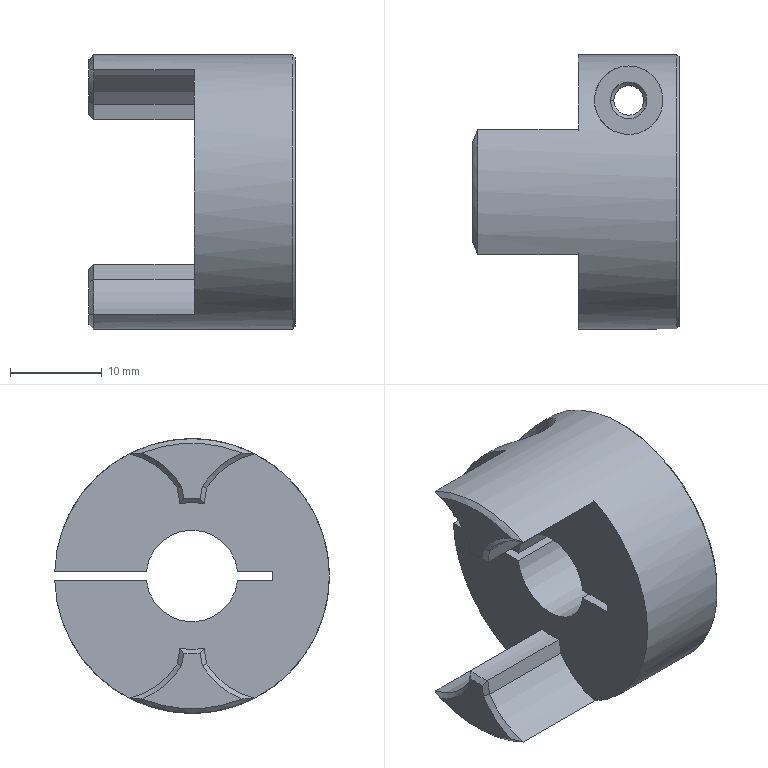Part | NX | 1 solid | 48 faces | box 22.5 x 29.992 x 30 mm | volume 7346 mm3 | plane 18 | cylinder 17 | cone 13 | commonest cylinder face diameters 4 x4 16.982 x4 3.242 x2 7.5 x2 10 x2 16 x2